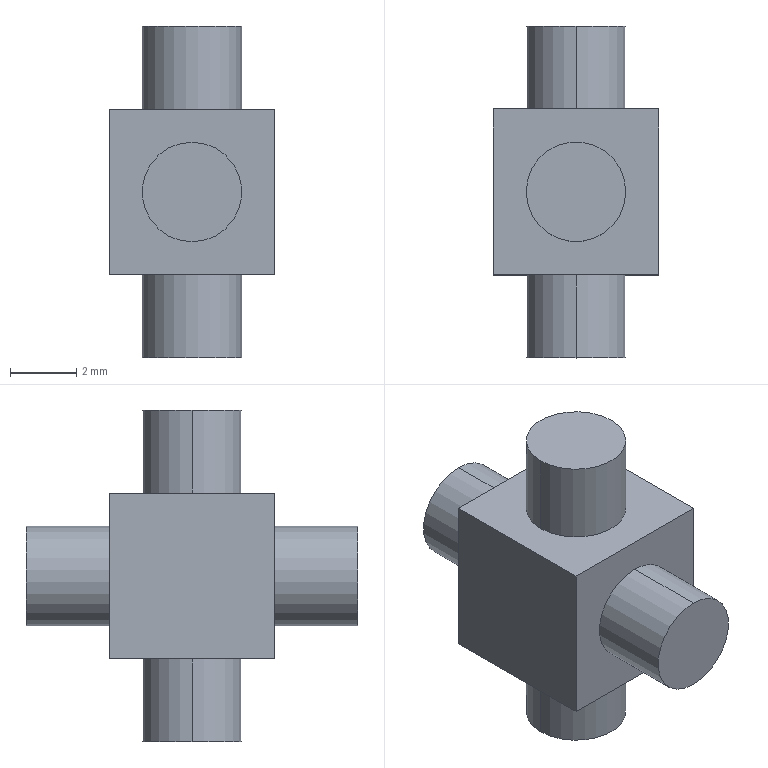Part | SolidWorks | features ICE 2, Extrusion 1 | 1 solid | 18 faces | box 5 x 10 x 10 mm | volume 195.686 mm3 | plane 10 | cylinder 8 | commonest cylinder face diameters 3 x8
STEP:
#1=CARTESIAN_POINT('',(1.5,0.,5.));
#2=VERTEX_POINT('',#1);
#3=CARTESIAN_POINT('',(-1.5,0.,5.));
#4=VERTEX_POINT('',#3);
#5=CARTESIAN_POINT('',(0.,0.,5.));
#6=DIRECTION('',(0.,0.,1.));
#7=DIRECTION('',(1.,0.,0.));
#8=AXIS2_PLACEMENT_3D('',#5,#6,#7);
#9=CIRCLE('',#8,1.5);
#10=EDGE_CURVE('',#2,#4,#9,.T.);
#11=ORIENTED_EDGE('',*,*,#10,.F.);
#12=CARTESIAN_POINT('',(1.5,0.,2.5));
#13=VERTEX_POINT('',#12);
#14=CARTESIAN_POINT('',(1.5,0.,5.));
#15=DIRECTION('',(0.,0.,-1.));
#16=VECTOR('',#15,1000.);
#17=LINE('',#14,#16);
#18=EDGE_CURVE('',#2,#13,#17,.T.);
#19=ORIENTED_EDGE('',*,*,#18,.T.);
#20=CARTESIAN_POINT('',(-1.5,0.,2.5));
#21=VERTEX_POINT('',#20);
#22=CARTESIAN_POINT('',(0.,0.,2.5));
#23=DIRECTION('',(0.,0.,-1.));
#24=DIRECTION('',(1.,0.,0.));
#25=AXIS2_PLACEMENT_3D('',#22,#23,#24);
#26=CIRCLE('',#25,1.5);
#27=EDGE_CURVE('',#21,#13,#26,.T.);
#28=ORIENTED_EDGE('',*,*,#27,.F.);
#29=CARTESIAN_POINT('',(-1.5,0.,5.));
#30=DIRECTION('',(0.,0.,-1.));
#31=VECTOR('',#30,1000.);
#32=LINE('',#29,#31);
#33=EDGE_CURVE('',#4,#21,#32,.T.);
#34=ORIENTED_EDGE('',*,*,#33,.F.);
#35=EDGE_LOOP('',(#11,#19,#28,#34));
#36=FACE_OUTER_BOUND('',#35,.T.);
#37=CARTESIAN_POINT('',(0.,0.,5.));
#38=DIRECTION('',(0.,0.,-1.));
#39=DIRECTION('',(-1.,0.,0.));
#40=AXIS2_PLACEMENT_3D('',#37,#38,#39);
#41=CYLINDRICAL_SURFACE('',#40,1.5);
#42=ADVANCED_FACE('',(#36),#41,.T.);
#43=CARTESIAN_POINT('',(-1.5,0.,-2.5));
#44=VERTEX_POINT('',#43);
#45=CARTESIAN_POINT('',(1.5,0.,-2.5));
#46=VERTEX_POINT('',#45);
#47=CARTESIAN_POINT('',(0.,0.,-2.5));
#48=DIRECTION('',(0.,0.,-1.));
#49=DIRECTION('',(1.,0.,0.));
#50=AXIS2_PLACEMENT_3D('',#47,#48,#49);
#51=CIRCLE('',#50,1.5);
#52=EDGE_CURVE('',#44,#46,#51,.T.);
#53=ORIENTED_EDGE('',*,*,#52,.T.);
#54=CARTESIAN_POINT('',(1.5,0.,-5.));
#55=VERTEX_POINT('',#54);
#56=CARTESIAN_POINT('',(1.5,0.,5.));
#57=DIRECTION('',(0.,0.,-1.));
#58=VECTOR('',#57,1000.);
#59=LINE('',#56,#58);
#60=EDGE_CURVE('',#46,#55,#59,.T.);
#61=ORIENTED_EDGE('',*,*,#60,.T.);
#62=CARTESIAN_POINT('',(-1.5,0.,-5.));
#63=VERTEX_POINT('',#62);
#64=CARTESIAN_POINT('',(0.,0.,-5.));
#65=DIRECTION('',(0.,0.,1.));
#66=DIRECTION('',(1.,0.,0.));
#67=AXIS2_PLACEMENT_3D('',#64,#65,#66);
#68=CIRCLE('',#67,1.5);
#69=EDGE_CURVE('',#55,#63,#68,.T.);
#70=ORIENTED_EDGE('',*,*,#69,.T.);
#71=CARTESIAN_POINT('',(-1.5,0.,5.));
#72=DIRECTION('',(0.,0.,-1.));
#73=VECTOR('',#72,1000.);
#74=LINE('',#71,#73);
#75=EDGE_CURVE('',#44,#63,#74,.T.);
#76=ORIENTED_EDGE('',*,*,#75,.F.);
#77=EDGE_LOOP('',(#53,#61,#70,#76));
#78=FACE_OUTER_BOUND('',#77,.T.);
#79=CARTESIAN_POINT('',(0.,0.,5.));
#80=DIRECTION('',(0.,0.,-1.));
#81=DIRECTION('',(-1.,0.,0.));
#82=AXIS2_PLACEMENT_3D('',#79,#80,#81);
#83=CYLINDRICAL_SURFACE('',#82,1.5);
#84=ADVANCED_FACE('',(#78),#83,.T.);
#85=CARTESIAN_POINT('',(0.,-2.5,-1.5));
#86=VERTEX_POINT('',#85);
#87=CARTESIAN_POINT('',(0.,-2.5,1.5));
#88=VERTEX_POINT('',#87);
#89=CARTESIAN_POINT('',(0.,-2.5,0.));
#90=DIRECTION('',(0.,-1.,0.));
#91=DIRECTION('',(0.,0.,1.));
#92=AXIS2_PLACEMENT_3D('',#89,#90,#91);
#93=CIRCLE('',#92,1.5);
#94=EDGE_CURVE('',#86,#88,#93,.T.);
#95=ORIENTED_EDGE('',*,*,#94,.T.);
#96=CARTESIAN_POINT('',(0.,-5.,1.5));
#97=VERTEX_POINT('',#96);
#98=CARTESIAN_POINT('',(0.,5.,1.5));
#99=DIRECTION('',(0.,-1.,0.));
#100=VECTOR('',#99,1000.);
#101=LINE('',#98,#100);
#102=EDGE_CURVE('',#88,#97,#101,.T.);
#103=ORIENTED_EDGE('',*,*,#102,.T.);
#104=CARTESIAN_POINT('',(0.,-5.,-1.5));
#105=VERTEX_POINT('',#104);
#106=CARTESIAN_POINT('',(0.,-5.,0.));
#107=DIRECTION('',(0.,1.,0.));
#108=DIRECTION('',(0.,0.,1.));
#109=AXIS2_PLACEMENT_3D('',#106,#107,#108);
#110=CIRCLE('',#109,1.5);
#111=EDGE_CURVE('',#97,#105,#110,.T.);
#112=ORIENTED_EDGE('',*,*,#111,.T.);
#113=CARTESIAN_POINT('',(0.,5.,-1.5));
#114=DIRECTION('',(0.,-1.,0.));
#115=VECTOR('',#114,1000.);
#116=LINE('',#113,#115);
#117=EDGE_CURVE('',#86,#105,#116,.T.);
#118=ORIENTED_EDGE('',*,*,#117,.F.);
#119=EDGE_LOOP('',(#95,#103,#112,#118));
#120=FACE_OUTER_BOUND('',#119,.T.);
#121=CARTESIAN_POINT('',(0.,5.,0.));
#122=DIRECTION('',(0.,-1.,0.));
#123=DIRECTION('',(0.,0.,-1.));
#124=AXIS2_PLACEMENT_3D('',#121,#122,#123);
#125=CYLINDRICAL_SURFACE('',#124,1.5);
#126=ADVANCED_FACE('',(#120),#125,.T.);
#127=CARTESIAN_POINT('',(0.,5.,1.5));
#128=VERTEX_POINT('',#127);
#129=CARTESIAN_POINT('',(0.,5.,-1.5));
#130=VERTEX_POINT('',#129);
#131=CARTESIAN_POINT('',(0.,5.,0.));
#132=DIRECTION('',(0.,1.,0.));
#133=DIRECTION('',(0.,0.,1.));
#134=AXIS2_PLACEMENT_3D('',#131,#132,#133);
#135=CIRCLE('',#134,1.5);
#136=EDGE_CURVE('',#128,#130,#135,.T.);
#137=ORIENTED_EDGE('',*,*,#136,.F.);
#138=CARTESIAN_POINT('',(0.,2.5,1.5));
#139=VERTEX_POINT('',#138);
#140=CARTESIAN_POINT('',(0.,5.,1.5));
#141=DIRECTION('',(0.,-1.,0.));
#142=VECTOR('',#141,1000.);
#143=LINE('',#140,#142);
#144=EDGE_CURVE('',#128,#139,#143,.T.);
#145=ORIENTED_EDGE('',*,*,#144,.T.);
#146=CARTESIAN_POINT('',(0.,2.5,-1.5));
#147=VERTEX_POINT('',#146);
#148=CARTESIAN_POINT('',(0.,2.5,0.));
#149=DIRECTION('',(0.,1.,0.));
#150=DIRECTION('',(0.,0.,-1.));
#151=AXIS2_PLACEMENT_3D('',#148,#149,#150);
#152=CIRCLE('',#151,1.5);
#153=EDGE_CURVE('',#139,#147,#152,.T.);
#154=ORIENTED_EDGE('',*,*,#153,.T.);
#155=CARTESIAN_POINT('',(0.,5.,-1.5));
#156=DIRECTION('',(0.,-1.,0.));
#157=VECTOR('',#156,1000.);
#158=LINE('',#155,#157);
#159=EDGE_CURVE('',#130,#147,#158,.T.);
#160=ORIENTED_EDGE('',*,*,#159,.F.);
#161=EDGE_LOOP('',(#137,#145,#154,#160));
#162=FACE_OUTER_BOUND('',#161,.T.);
#163=CARTESIAN_POINT('',(0.,5.,0.));
#164=DIRECTION('',(0.,-1.,0.));
#165=DIRECTION('',(0.,0.,-1.));
#166=AXIS2_PLACEMENT_3D('',#163,#164,#165);
#167=CYLINDRICAL_SURFACE('',#166,1.5);
#168=ADVANCED_FACE('',(#162),#167,.T.);
#169=CARTESIAN_POINT('',(-2.5,2.5,-2.5));
#170=VERTEX_POINT('',#169);
#171=CARTESIAN_POINT('',(-2.5,-2.5,-2.5));
#172=VERTEX_POINT('',#171);
#173=CARTESIAN_POINT('',(-2.5,2.5,-2.5));
#174=DIRECTION('',(0.,-1.,0.));
#175=VECTOR('',#174,1000.);
#176=LINE('',#173,#175);
#177=EDGE_CURVE('',#170,#172,#176,.T.);
#178=ORIENTED_EDGE('',*,*,#177,.T.);
#179=CARTESIAN_POINT('',(-2.5,-2.5,2.5));
#180=VERTEX_POINT('',#179);
#181=CARTESIAN_POINT('',(-2.5,-2.5,2.5));
#182=DIRECTION('',(0.,0.,-1.));
#183=VECTOR('',#182,1000.);
#184=LINE('',#181,#183);
#185=EDGE_CURVE('',#180,#172,#184,.T.);
#186=ORIENTED_EDGE('',*,*,#185,.F.);
#187=CARTESIAN_POINT('',(-2.5,2.5,2.5));
#188=VERTEX_POINT('',#187);
#189=CARTESIAN_POINT('',(-2.5,2.5,2.5));
#190=DIRECTION('',(0.,-1.,0.));
#191=VECTOR('',#190,1000.);
#192=LINE('',#189,#191);
#193=EDGE_CURVE('',#188,#180,#192,.T.);
#194=ORIENTED_EDGE('',*,*,#193,.F.);
#195=CARTESIAN_POINT('',(-2.5,2.5,2.5));
#196=DIRECTION('',(0.,0.,-1.));
#197=VECTOR('',#196,1000.);
#198=LINE('',#195,#197);
#199=EDGE_CURVE('',#188,#170,#198,.T.);
#200=ORIENTED_EDGE('',*,*,#199,.T.);
#201=EDGE_LOOP('',(#178,#186,#194,#200));
#202=FACE_OUTER_BOUND('',#201,.T.);
#203=CARTESIAN_POINT('',(-2.5,2.5,2.5));
#204=DIRECTION('',(1.,0.,0.));
#205=DIRECTION('',(0.,0.,-1.));
#206=AXIS2_PLACEMENT_3D('',#203,#204,#205);
#207=PLANE('',#206);
#208=ADVANCED_FACE('',(#202),#207,.F.);
#209=ORIENTED_EDGE('',*,*,#94,.F.);
#210=CARTESIAN_POINT('',(0.,-2.5,0.));
#211=DIRECTION('',(0.,-1.,0.));
#212=DIRECTION('',(0.,0.,1.));
#213=AXIS2_PLACEMENT_3D('',#210,#211,#212);
#214=CIRCLE('',#213,1.5);
#215=EDGE_CURVE('',#88,#86,#214,.T.);
#216=ORIENTED_EDGE('',*,*,#215,.F.);
#217=EDGE_LOOP('',(#209,#216));
#218=FACE_BOUND('',#217,.T.);
#219=CARTESIAN_POINT('',(2.5,-2.5,-2.5));
#220=VERTEX_POINT('',#219);
#221=CARTESIAN_POINT('',(-2.5,-2.5,-2.5));
#222=DIRECTION('',(1.,0.,0.));
#223=VECTOR('',#222,1000.);
#224=LINE('',#221,#223);
#225=EDGE_CURVE('',#172,#220,#224,.T.);
#226=ORIENTED_EDGE('',*,*,#225,.T.);
#227=CARTESIAN_POINT('',(2.5,-2.5,2.5));
#228=VERTEX_POINT('',#227);
#229=CARTESIAN_POINT('',(2.5,-2.5,2.5));
#230=DIRECTION('',(0.,0.,-1.));
#231=VECTOR('',#230,1000.);
#232=LINE('',#229,#231);
#233=EDGE_CURVE('',#228,#220,#232,.T.);
#234=ORIENTED_EDGE('',*,*,#233,.F.);
#235=CARTESIAN_POINT('',(-2.5,-2.5,2.5));
#236=DIRECTION('',(1.,0.,0.));
#237=VECTOR('',#236,1000.);
#238=LINE('',#235,#237);
#239=EDGE_CURVE('',#180,#228,#238,.T.);
#240=ORIENTED_EDGE('',*,*,#239,.F.);
#241=ORIENTED_EDGE('',*,*,#185,.T.);
#242=EDGE_LOOP('',(#226,#234,#240,#241));
#243=FACE_OUTER_BOUND('',#242,.T.);
#244=CARTESIAN_POINT('',(-2.5,-2.5,2.5));
#245=DIRECTION('',(0.,1.,0.));
#246=DIRECTION('',(0.,0.,1.));
#247=AXIS2_PLACEMENT_3D('',#244,#245,#246);
#248=PLANE('',#247);
#249=ADVANCED_FACE('',(#218,#243),#248,.F.);
#250=CARTESIAN_POINT('',(2.5,2.5,-2.5));
#251=VERTEX_POINT('',#250);
#252=CARTESIAN_POINT('',(2.5,2.5,-2.5));
#253=DIRECTION('',(0.,1.,0.));
#254=VECTOR('',#253,1000.);
#255=LINE('',#252,#254);
#256=EDGE_CURVE('',#220,#251,#255,.T.);
#257=ORIENTED_EDGE('',*,*,#256,.T.);
#258=CARTESIAN_POINT('',(2.5,2.5,2.5));
#259=VERTEX_POINT('',#258);
#260=CARTESIAN_POINT('',(2.5,2.5,2.5));
#261=DIRECTION('',(0.,0.,-1.));
#262=VECTOR('',#261,1000.);
#263=LINE('',#260,#262);
#264=EDGE_CURVE('',#259,#251,#263,.T.);
#265=ORIENTED_EDGE('',*,*,#264,.F.);
#266=CARTESIAN_POINT('',(2.5,2.5,2.5));
#267=DIRECTION('',(0.,1.,0.));
#268=VECTOR('',#267,1000.);
#269=LINE('',#266,#268);
#270=EDGE_CURVE('',#228,#259,#269,.T.);
#271=ORIENTED_EDGE('',*,*,#270,.F.);
#272=ORIENTED_EDGE('',*,*,#233,.T.);
#273=EDGE_LOOP('',(#257,#265,#271,#272));
#274=FACE_OUTER_BOUND('',#273,.T.);
#275=CARTESIAN_POINT('',(2.5,2.5,2.5));
#276=DIRECTION('',(-1.,0.,0.));
#277=DIRECTION('',(0.,0.,1.));
#278=AXIS2_PLACEMENT_3D('',#275,#276,#277);
#279=PLANE('',#278);
#280=ADVANCED_FACE('',(#274),#279,.F.);
#281=CARTESIAN_POINT('',(0.,2.5,0.));
#282=DIRECTION('',(0.,1.,0.));
#283=DIRECTION('',(0.,0.,-1.));
#284=AXIS2_PLACEMENT_3D('',#281,#282,#283);
#285=CIRCLE('',#284,1.5);
#286=EDGE_CURVE('',#147,#139,#285,.T.);
#287=ORIENTED_EDGE('',*,*,#286,.F.);
#288=ORIENTED_EDGE('',*,*,#153,.F.);
#289=EDGE_LOOP('',(#287,#288));
#290=FACE_BOUND('',#289,.T.);
#291=CARTESIAN_POINT('',(-2.5,2.5,-2.5));
#292=DIRECTION('',(-1.,0.,0.));
#293=VECTOR('',#292,1000.);
#294=LINE('',#291,#293);
#295=EDGE_CURVE('',#251,#170,#294,.T.);
#296=ORIENTED_EDGE('',*,*,#295,.T.);
#297=ORIENTED_EDGE('',*,*,#199,.F.);
#298=CARTESIAN_POINT('',(-2.5,2.5,2.5));
#299=DIRECTION('',(-1.,0.,0.));
#300=VECTOR('',#299,1000.);
#301=LINE('',#298,#300);
#302=EDGE_CURVE('',#259,#188,#301,.T.);
#303=ORIENTED_EDGE('',*,*,#302,.F.);
#304=ORIENTED_EDGE('',*,*,#264,.T.);
#305=EDGE_LOOP('',(#296,#297,#303,#304));
#306=FACE_OUTER_BOUND('',#305,.T.);
#307=CARTESIAN_POINT('',(-2.5,2.5,2.5));
#308=DIRECTION('',(0.,-1.,0.));
#309=DIRECTION('',(0.,0.,-1.));
#310=AXIS2_PLACEMENT_3D('',#307,#308,#309);
#311=PLANE('',#310);
#312=ADVANCED_FACE('',(#290,#306),#311,.F.);
#313=ORIENTED_EDGE('',*,*,#27,.T.);
#314=CARTESIAN_POINT('',(0.,0.,2.5));
#315=DIRECTION('',(0.,0.,-1.));
#316=DIRECTION('',(1.,0.,0.));
#317=AXIS2_PLACEMENT_3D('',#314,#315,#316);
#318=CIRCLE('',#317,1.5);
#319=EDGE_CURVE('',#13,#21,#318,.T.);
#320=ORIENTED_EDGE('',*,*,#319,.T.);
#321=EDGE_LOOP('',(#313,#320));
#322=FACE_BOUND('',#321,.T.);
#323=ORIENTED_EDGE('',*,*,#193,.T.);
#324=ORIENTED_EDGE('',*,*,#239,.T.);
#325=ORIENTED_EDGE('',*,*,#270,.T.);
#326=ORIENTED_EDGE('',*,*,#302,.T.);
#327=EDGE_LOOP('',(#323,#324,#325,#326));
#328=FACE_OUTER_BOUND('',#327,.T.);
#329=CARTESIAN_POINT('',(0.,0.,2.5));
#330=DIRECTION('',(0.,0.,1.));
#331=DIRECTION('',(1.,0.,0.));
#332=AXIS2_PLACEMENT_3D('',#329,#330,#331);
#333=PLANE('',#332);
#334=ADVANCED_FACE('',(#322,#328),#333,.T.);
#335=ORIENTED_EDGE('',*,*,#52,.F.);
#336=CARTESIAN_POINT('',(0.,0.,-2.5));
#337=DIRECTION('',(0.,0.,-1.));
#338=DIRECTION('',(1.,0.,0.));
#339=AXIS2_PLACEMENT_3D('',#336,#337,#338);
#340=CIRCLE('',#339,1.5);
#341=EDGE_CURVE('',#46,#44,#340,.T.);
#342=ORIENTED_EDGE('',*,*,#341,.F.);
#343=EDGE_LOOP('',(#335,#342));
#344=FACE_BOUND('',#343,.T.);
#345=ORIENTED_EDGE('',*,*,#177,.F.);
#346=ORIENTED_EDGE('',*,*,#295,.F.);
#347=ORIENTED_EDGE('',*,*,#256,.F.);
#348=ORIENTED_EDGE('',*,*,#225,.F.);
#349=EDGE_LOOP('',(#345,#346,#347,#348));
#350=FACE_OUTER_BOUND('',#349,.T.);
#351=CARTESIAN_POINT('',(0.,0.,-2.5));
#352=DIRECTION('',(0.,0.,1.));
#353=DIRECTION('',(1.,0.,0.));
#354=AXIS2_PLACEMENT_3D('',#351,#352,#353);
#355=PLANE('',#354);
#356=ADVANCED_FACE('',(#344,#350),#355,.F.);
#357=CARTESIAN_POINT('',(0.,5.,0.));
#358=DIRECTION('',(0.,1.,0.));
#359=DIRECTION('',(0.,0.,1.));
#360=AXIS2_PLACEMENT_3D('',#357,#358,#359);
#361=CIRCLE('',#360,1.5);
#362=EDGE_CURVE('',#130,#128,#361,.T.);
#363=ORIENTED_EDGE('',*,*,#362,.T.);
#364=ORIENTED_EDGE('',*,*,#136,.T.);
#365=EDGE_LOOP('',(#363,#364));
#366=FACE_OUTER_BOUND('',#365,.T.);
#367=CARTESIAN_POINT('',(0.,5.,0.));
#368=DIRECTION('',(0.,1.,0.));
#369=DIRECTION('',(0.,0.,1.));
#370=AXIS2_PLACEMENT_3D('',#367,#368,#369);
#371=PLANE('',#370);
#372=ADVANCED_FACE('',(#366),#371,.T.);
#373=ORIENTED_EDGE('',*,*,#144,.F.);
#374=ORIENTED_EDGE('',*,*,#362,.F.);
#375=ORIENTED_EDGE('',*,*,#159,.T.);
#376=ORIENTED_EDGE('',*,*,#286,.T.);
#377=EDGE_LOOP('',(#373,#374,#375,#376));
#378=FACE_OUTER_BOUND('',#377,.T.);
#379=CARTESIAN_POINT('',(0.,5.,0.));
#380=DIRECTION('',(0.,-1.,0.));
#381=DIRECTION('',(0.,0.,-1.));
#382=AXIS2_PLACEMENT_3D('',#379,#380,#381);
#383=CYLINDRICAL_SURFACE('',#382,1.5);
#384=ADVANCED_FACE('',(#378),#383,.T.);
#385=ORIENTED_EDGE('',*,*,#102,.F.);
#386=ORIENTED_EDGE('',*,*,#215,.T.);
#387=ORIENTED_EDGE('',*,*,#117,.T.);
#388=CARTESIAN_POINT('',(0.,-5.,0.));
#389=DIRECTION('',(0.,1.,0.));
#390=DIRECTION('',(0.,0.,1.));
#391=AXIS2_PLACEMENT_3D('',#388,#389,#390);
#392=CIRCLE('',#391,1.5);
#393=EDGE_CURVE('',#105,#97,#392,.T.);
#394=ORIENTED_EDGE('',*,*,#393,.T.);
#395=EDGE_LOOP('',(#385,#386,#387,#394));
#396=FACE_OUTER_BOUND('',#395,.T.);
#397=CARTESIAN_POINT('',(0.,5.,0.));
#398=DIRECTION('',(0.,-1.,0.));
#399=DIRECTION('',(0.,0.,-1.));
#400=AXIS2_PLACEMENT_3D('',#397,#398,#399);
#401=CYLINDRICAL_SURFACE('',#400,1.5);
#402=ADVANCED_FACE('',(#396),#401,.T.);
#403=ORIENTED_EDGE('',*,*,#393,.F.);
#404=ORIENTED_EDGE('',*,*,#111,.F.);
#405=EDGE_LOOP('',(#403,#404));
#406=FACE_OUTER_BOUND('',#405,.T.);
#407=CARTESIAN_POINT('',(0.,-5.,0.));
#408=DIRECTION('',(0.,1.,0.));
#409=DIRECTION('',(0.,0.,1.));
#410=AXIS2_PLACEMENT_3D('',#407,#408,#409);
#411=PLANE('',#410);
#412=ADVANCED_FACE('',(#406),#411,.F.);
#413=CARTESIAN_POINT('',(0.,0.,-5.));
#414=DIRECTION('',(0.,0.,1.));
#415=DIRECTION('',(1.,0.,0.));
#416=AXIS2_PLACEMENT_3D('',#413,#414,#415);
#417=CIRCLE('',#416,1.5);
#418=EDGE_CURVE('',#63,#55,#417,.T.);
#419=ORIENTED_EDGE('',*,*,#418,.F.);
#420=ORIENTED_EDGE('',*,*,#69,.F.);
#421=EDGE_LOOP('',(#419,#420));
#422=FACE_OUTER_BOUND('',#421,.T.);
#423=CARTESIAN_POINT('',(0.,0.,-5.));
#424=DIRECTION('',(0.,0.,1.));
#425=DIRECTION('',(1.,0.,0.));
#426=AXIS2_PLACEMENT_3D('',#423,#424,#425);
#427=PLANE('',#426);
#428=ADVANCED_FACE('',(#422),#427,.F.);
#429=ORIENTED_EDGE('',*,*,#60,.F.);
#430=ORIENTED_EDGE('',*,*,#341,.T.);
#431=ORIENTED_EDGE('',*,*,#75,.T.);
#432=ORIENTED_EDGE('',*,*,#418,.T.);
#433=EDGE_LOOP('',(#429,#430,#431,#432));
#434=FACE_OUTER_BOUND('',#433,.T.);
#435=CARTESIAN_POINT('',(0.,0.,5.));
#436=DIRECTION('',(0.,0.,-1.));
#437=DIRECTION('',(-1.,0.,0.));
#438=AXIS2_PLACEMENT_3D('',#435,#436,#437);
#439=CYLINDRICAL_SURFACE('',#438,1.5);
#440=ADVANCED_FACE('',(#434),#439,.T.);
#441=ORIENTED_EDGE('',*,*,#18,.F.);
#442=CARTESIAN_POINT('',(0.,0.,5.));
#443=DIRECTION('',(0.,0.,1.));
#444=DIRECTION('',(1.,0.,0.));
#445=AXIS2_PLACEMENT_3D('',#442,#443,#444);
#446=CIRCLE('',#445,1.5);
#447=EDGE_CURVE('',#4,#2,#446,.T.);
#448=ORIENTED_EDGE('',*,*,#447,.F.);
#449=ORIENTED_EDGE('',*,*,#33,.T.);
#450=ORIENTED_EDGE('',*,*,#319,.F.);
#451=EDGE_LOOP('',(#441,#448,#449,#450));
#452=FACE_OUTER_BOUND('',#451,.T.);
#453=CARTESIAN_POINT('',(0.,0.,5.));
#454=DIRECTION('',(0.,0.,-1.));
#455=DIRECTION('',(-1.,0.,0.));
#456=AXIS2_PLACEMENT_3D('',#453,#454,#455);
#457=CYLINDRICAL_SURFACE('',#456,1.5);
#458=ADVANCED_FACE('',(#452),#457,.T.);
#459=ORIENTED_EDGE('',*,*,#447,.T.);
#460=ORIENTED_EDGE('',*,*,#10,.T.);
#461=EDGE_LOOP('',(#459,#460));
#462=FACE_OUTER_BOUND('',#461,.T.);
#463=CARTESIAN_POINT('',(0.,0.,5.));
#464=DIRECTION('',(0.,0.,1.));
#465=DIRECTION('',(1.,0.,0.));
#466=AXIS2_PLACEMENT_3D('',#463,#464,#465);
#467=PLANE('',#466);
#468=ADVANCED_FACE('',(#462),#467,.T.);
#469=CLOSED_SHELL('',(#42,#84,#126,#168,#208,#249,#280,#312,#334,#356,#372,#384,#402,#412,#428,#440,#458,#468));
#470=MANIFOLD_SOLID_BREP('',#469);
#471=CARTESIAN_POINT('',(0.,0.,0.));
#472=DIRECTION('',(0.,0.,1.));
#473=DIRECTION('',(1.,0.,0.));
#474=AXIS2_PLACEMENT_3D('',#471,#472,#473);
#475=(LENGTH_UNIT()NAMED_UNIT(*)SI_UNIT(.MILLI.,.METRE.));
#476=UNCERTAINTY_MEASURE_WITH_UNIT(LENGTH_MEASURE(0.00001),#475,'','');
#477=(NAMED_UNIT(*)PLANE_ANGLE_UNIT()SI_UNIT($,.RADIAN.));
#478=(NAMED_UNIT(*)SI_UNIT($,.STERADIAN.)SOLID_ANGLE_UNIT());
#479=(GEOMETRIC_REPRESENTATION_CONTEXT(3)GLOBAL_UNCERTAINTY_ASSIGNED_CONTEXT((#476))GLOBAL_UNIT_ASSIGNED_CONTEXT((#475,#477,#478))REPRESENTATION_CONTEXT('',''));
#480=ADVANCED_BREP_SHAPE_REPRESENTATION('',(#470,#474),#479);